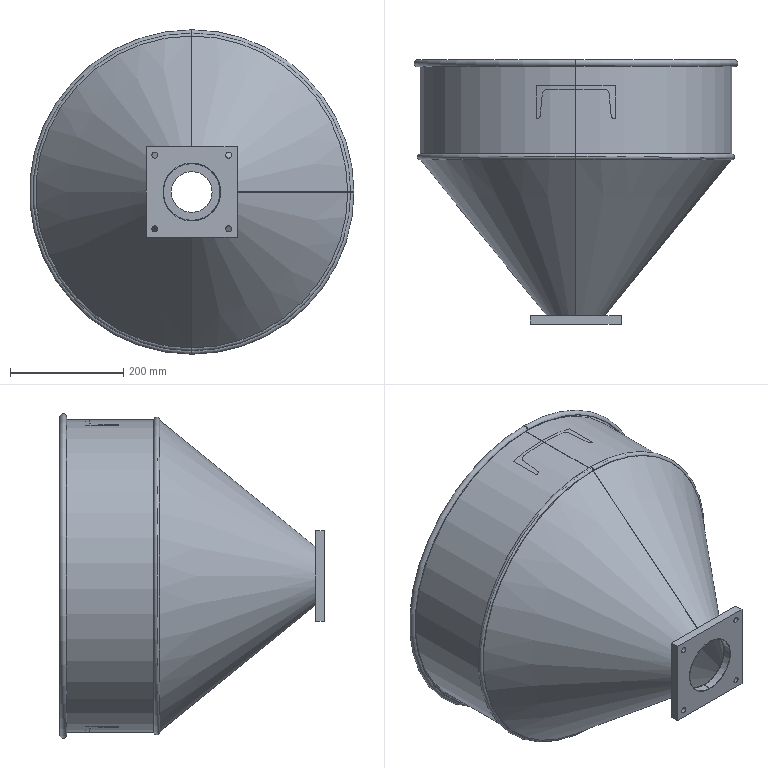Part | SolidWorks | features BaseBody 4 | 4 solids | 107 faces | box 572 x 466.152 x 572 mm | volume 1942635 mm3 | cylinder 44 | plane 30 | torus 24 | cone 9 | commonest cylinder face diameters 10.5 x8 12 x8 550 x6 102 x5 548 x5 100 x3